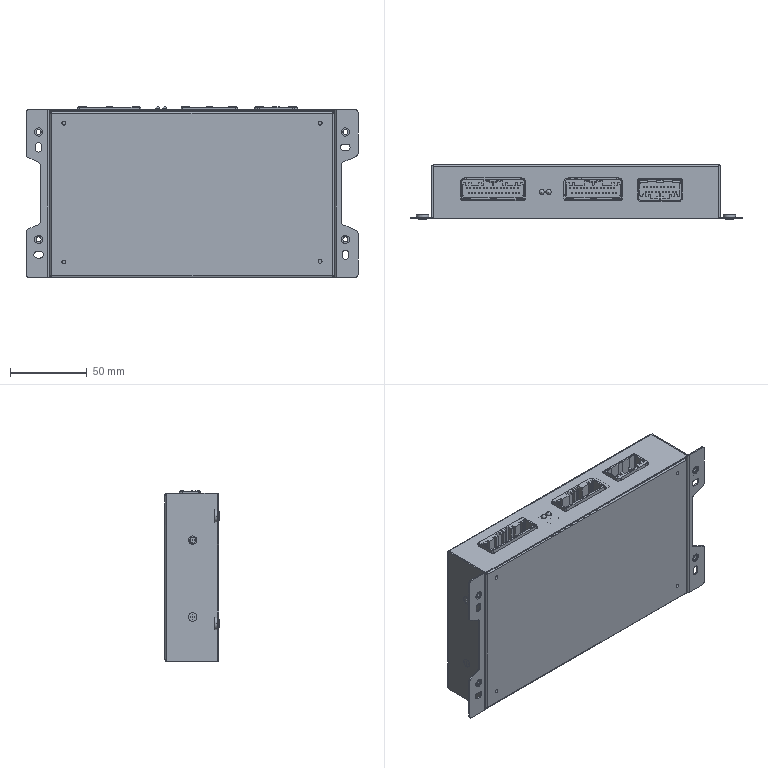Part | SolidWorks | 27 solids | 3967 faces | volume 121145 mm3 | plane 2012 | cylinder 1879 | cone 52 | spline 22 | sphere 2 | commonest cylinder face diameters 0.305 x670 0.6 x192 0.381 x136 0.7 x120 1 x110 0.889 x104